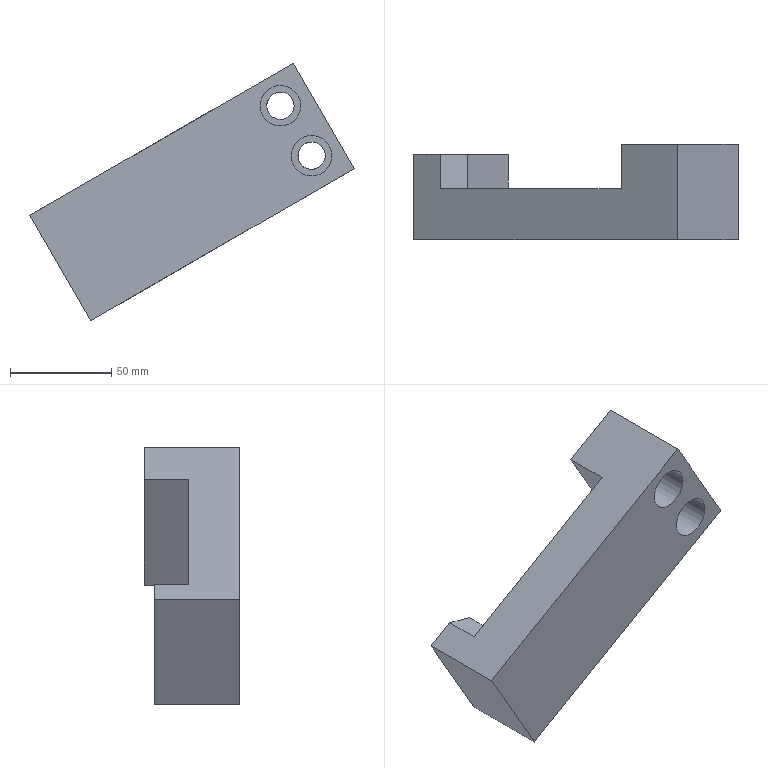Part | NX | features solid 2 | 1 solid | 18 faces | box 159.904 x 47 x 126.962 mm | volume 272454 mm3 | plane 14 | cylinder 4 | commonest cylinder face diameters 13.5 x2 20 x2
STEP:
#1=CARTESIAN_POINT('',(-1100.271,-395.,1.637));
#2=VERTEX_POINT('',#1);
#3=CARTESIAN_POINT('',(-1011.07,-395.,53.137));
#4=VERTEX_POINT('',#3);
#5=CARTESIAN_POINT('',(-1005.874,-395.,56.137));
#6=DIRECTION('',(0.866,0.,0.5));
#7=VECTOR('',#6,1000.);
#8=LINE('',#5,#7);
#9=EDGE_CURVE('',#2,#4,#8,.T.);
#10=ORIENTED_EDGE('',*,*,#9,.T.);
#11=CARTESIAN_POINT('',(-981.07,-395.,1.176));
#12=VERTEX_POINT('',#11);
#13=CARTESIAN_POINT('',(-983.42,-395.,5.246));
#14=DIRECTION('',(-0.5,0.,0.866));
#15=VECTOR('',#14,1000.);
#16=LINE('',#13,#15);
#17=EDGE_CURVE('',#12,#4,#16,.T.);
#18=ORIENTED_EDGE('',*,*,#17,.F.);
#19=CARTESIAN_POINT('',(-1070.271,-395.,-50.324));
#20=VERTEX_POINT('',#19);
#21=CARTESIAN_POINT('',(-975.874,-395.,4.176));
#22=DIRECTION('',(0.866,0.,0.5));
#23=VECTOR('',#22,1000.);
#24=LINE('',#21,#23);
#25=EDGE_CURVE('',#20,#12,#24,.T.);
#26=ORIENTED_EDGE('',*,*,#25,.F.);
#27=CARTESIAN_POINT('',(-1066.61,-395.,-36.664));
#28=VERTEX_POINT('',#27);
#29=CARTESIAN_POINT('',(-1049.462,-395.,27.334));
#30=DIRECTION('',(0.2588,0.,0.9659));
#31=VECTOR('',#30,1000.);
#32=LINE('',#29,#31);
#33=EDGE_CURVE('',#20,#28,#32,.T.);
#34=ORIENTED_EDGE('',*,*,#33,.T.);
#35=CARTESIAN_POINT('',(-1086.61,-395.,-2.023));
#36=VERTEX_POINT('',#35);
#37=CARTESIAN_POINT('',(-1063.96,-395.,-41.254));
#38=DIRECTION('',(-0.5,0.,0.866));
#39=VECTOR('',#38,1000.);
#40=LINE('',#37,#39);
#41=EDGE_CURVE('',#28,#36,#40,.T.);
#42=ORIENTED_EDGE('',*,*,#41,.T.);
#43=CARTESIAN_POINT('',(-988.052,-395.,-28.432));
#44=DIRECTION('',(0.9659,0.,-0.2588));
#45=VECTOR('',#44,1000.);
#46=LINE('',#43,#45);
#47=EDGE_CURVE('',#36,#2,#46,.F.);
#48=ORIENTED_EDGE('',*,*,#47,.T.);
#49=EDGE_LOOP('',(#10,#18,#26,#34,#42,#48));
#50=FACE_BOUND('',#49,.T.);
#51=CARTESIAN_POINT('',(-978.224,-395.,8.246));
#52=DIRECTION('',(0.,1.,0.));
#53=DIRECTION('',(-0.5,0.,0.866));
#54=AXIS2_PLACEMENT_3D('',#51,#52,#53);
#55=PLANE('',#54);
#56=ADVANCED_FACE('',(#50),#55,.T.);
#57=ORIENTED_EDGE('',*,*,#9,.F.);
#58=CARTESIAN_POINT('',(-1100.271,-378.,1.637));
#59=VERTEX_POINT('',#58);
#60=CARTESIAN_POINT('',(-1100.271,-335.,1.637));
#61=DIRECTION('',(0.,-1.,0.));
#62=VECTOR('',#61,1000.);
#63=LINE('',#60,#62);
#64=EDGE_CURVE('',#2,#59,#63,.F.);
#65=ORIENTED_EDGE('',*,*,#64,.T.);
#66=CARTESIAN_POINT('',(-1113.261,-378.,-5.863));
#67=VERTEX_POINT('',#66);
#68=CARTESIAN_POINT('',(-1100.271,-378.,1.637));
#69=DIRECTION('',(0.866,0.,0.5));
#70=VECTOR('',#69,1000.);
#71=LINE('',#68,#70);
#72=EDGE_CURVE('',#67,#59,#71,.T.);
#73=ORIENTED_EDGE('',*,*,#72,.F.);
#74=CARTESIAN_POINT('',(-1113.261,-420.,-5.863));
#75=VERTEX_POINT('',#74);
#76=CARTESIAN_POINT('',(-1113.261,-335.,-5.863));
#77=DIRECTION('',(0.,-1.,0.));
#78=VECTOR('',#77,1000.);
#79=LINE('',#76,#78);
#80=EDGE_CURVE('',#67,#75,#79,.T.);
#81=ORIENTED_EDGE('',*,*,#80,.T.);
#82=CARTESIAN_POINT('',(-983.357,-420.,69.137));
#83=VERTEX_POINT('',#82);
#84=CARTESIAN_POINT('',(-1096.807,-420.,3.637));
#85=DIRECTION('',(0.866,0.,0.5));
#86=VECTOR('',#85,1000.);
#87=LINE('',#84,#86);
#88=EDGE_CURVE('',#75,#83,#87,.T.);
#89=ORIENTED_EDGE('',*,*,#88,.T.);
#90=CARTESIAN_POINT('',(-983.357,-373.,69.137));
#91=VERTEX_POINT('',#90);
#92=CARTESIAN_POINT('',(-983.357,-370.,69.137));
#93=DIRECTION('',(0.,1.,0.));
#94=VECTOR('',#93,1000.);
#95=LINE('',#92,#94);
#96=EDGE_CURVE('',#83,#91,#95,.T.);
#97=ORIENTED_EDGE('',*,*,#96,.T.);
#98=CARTESIAN_POINT('',(-1011.07,-373.,53.137));
#99=VERTEX_POINT('',#98);
#100=CARTESIAN_POINT('',(-1096.807,-373.,3.637));
#101=DIRECTION('',(-0.866,0.,-0.5));
#102=VECTOR('',#101,1000.);
#103=LINE('',#100,#102);
#104=EDGE_CURVE('',#91,#99,#103,.T.);
#105=ORIENTED_EDGE('',*,*,#104,.T.);
#106=CARTESIAN_POINT('',(-1011.07,-335.,53.137));
#107=DIRECTION('',(0.,-1.,0.));
#108=VECTOR('',#107,1000.);
#109=LINE('',#106,#108);
#110=EDGE_CURVE('',#99,#4,#109,.T.);
#111=ORIENTED_EDGE('',*,*,#110,.T.);
#112=EDGE_LOOP('',(#57,#65,#73,#81,#89,#97,#105,#111));
#113=FACE_BOUND('',#112,.T.);
#114=CARTESIAN_POINT('',(-1096.807,-335.,3.637));
#115=DIRECTION('',(-0.5,0.,0.866));
#116=DIRECTION('',(0.866,0.,0.5));
#117=AXIS2_PLACEMENT_3D('',#114,#115,#116);
#118=PLANE('',#117);
#119=ADVANCED_FACE('',(#113),#118,.T.);
#120=ORIENTED_EDGE('',*,*,#72,.T.);
#121=CARTESIAN_POINT('',(-1086.61,-378.,-2.023));
#122=VERTEX_POINT('',#121);
#123=CARTESIAN_POINT('',(-1062.5,-378.,-8.484));
#124=DIRECTION('',(-0.9659,0.,0.2588));
#125=VECTOR('',#124,1000.);
#126=LINE('',#123,#125);
#127=EDGE_CURVE('',#59,#122,#126,.F.);
#128=ORIENTED_EDGE('',*,*,#127,.T.);
#129=CARTESIAN_POINT('',(-1066.61,-378.,-36.664));
#130=VERTEX_POINT('',#129);
#131=CARTESIAN_POINT('',(-1063.96,-378.,-41.254));
#132=DIRECTION('',(-0.5,0.,0.866));
#133=VECTOR('',#132,1000.);
#134=LINE('',#131,#133);
#135=EDGE_CURVE('',#130,#122,#134,.T.);
#136=ORIENTED_EDGE('',*,*,#135,.F.);
#137=CARTESIAN_POINT('',(-1070.271,-378.,-50.324));
#138=VERTEX_POINT('',#137);
#139=CARTESIAN_POINT('',(-1069.411,-378.,-47.114));
#140=DIRECTION('',(-0.2588,0.,-0.9659));
#141=VECTOR('',#140,1000.);
#142=LINE('',#139,#141);
#143=EDGE_CURVE('',#130,#138,#142,.T.);
#144=ORIENTED_EDGE('',*,*,#143,.T.);
#145=CARTESIAN_POINT('',(-1083.261,-378.,-57.824));
#146=VERTEX_POINT('',#145);
#147=CARTESIAN_POINT('',(-1070.271,-378.,-50.324));
#148=DIRECTION('',(0.866,0.,0.5));
#149=VECTOR('',#148,1000.);
#150=LINE('',#147,#149);
#151=EDGE_CURVE('',#146,#138,#150,.T.);
#152=ORIENTED_EDGE('',*,*,#151,.F.);
#153=CARTESIAN_POINT('',(-1085.611,-378.,-53.754));
#154=DIRECTION('',(-0.5,0.,0.866));
#155=VECTOR('',#154,1000.);
#156=LINE('',#153,#155);
#157=EDGE_CURVE('',#146,#67,#156,.T.);
#158=ORIENTED_EDGE('',*,*,#157,.T.);
#159=EDGE_LOOP('',(#120,#128,#136,#144,#152,#158));
#160=FACE_BOUND('',#159,.T.);
#161=CARTESIAN_POINT('',(-1072.621,-378.,-46.254));
#162=DIRECTION('',(0.,1.,0.));
#163=DIRECTION('',(0.342,0.,0.9397));
#164=AXIS2_PLACEMENT_3D('',#161,#162,#163);
#165=PLANE('',#164);
#166=ADVANCED_FACE('',(#160),#165,.T.);
#167=ORIENTED_EDGE('',*,*,#151,.T.);
#168=CARTESIAN_POINT('',(-1070.271,-335.,-50.324));
#169=DIRECTION('',(0.,-1.,0.));
#170=VECTOR('',#169,1000.);
#171=LINE('',#168,#170);
#172=EDGE_CURVE('',#138,#20,#171,.T.);
#173=ORIENTED_EDGE('',*,*,#172,.T.);
#174=ORIENTED_EDGE('',*,*,#25,.T.);
#175=CARTESIAN_POINT('',(-981.07,-373.,1.176));
#176=VERTEX_POINT('',#175);
#177=CARTESIAN_POINT('',(-981.07,-335.,1.176));
#178=DIRECTION('',(0.,-1.,0.));
#179=VECTOR('',#178,1000.);
#180=LINE('',#177,#179);
#181=EDGE_CURVE('',#176,#12,#180,.T.);
#182=ORIENTED_EDGE('',*,*,#181,.F.);
#183=CARTESIAN_POINT('',(-953.357,-373.,17.176));
#184=VERTEX_POINT('',#183);
#185=CARTESIAN_POINT('',(-1066.807,-373.,-48.324));
#186=DIRECTION('',(-0.866,0.,-0.5));
#187=VECTOR('',#186,1000.);
#188=LINE('',#185,#187);
#189=EDGE_CURVE('',#184,#176,#188,.T.);
#190=ORIENTED_EDGE('',*,*,#189,.F.);
#191=CARTESIAN_POINT('',(-953.357,-420.,17.176));
#192=VERTEX_POINT('',#191);
#193=CARTESIAN_POINT('',(-953.357,-370.,17.176));
#194=DIRECTION('',(0.,1.,0.));
#195=VECTOR('',#194,1000.);
#196=LINE('',#193,#195);
#197=EDGE_CURVE('',#192,#184,#196,.T.);
#198=ORIENTED_EDGE('',*,*,#197,.F.);
#199=CARTESIAN_POINT('',(-1083.261,-420.,-57.824));
#200=VERTEX_POINT('',#199);
#201=CARTESIAN_POINT('',(-1066.807,-420.,-48.324));
#202=DIRECTION('',(0.866,0.,0.5));
#203=VECTOR('',#202,1000.);
#204=LINE('',#201,#203);
#205=EDGE_CURVE('',#200,#192,#204,.T.);
#206=ORIENTED_EDGE('',*,*,#205,.F.);
#207=CARTESIAN_POINT('',(-1083.261,-335.,-57.824));
#208=DIRECTION('',(0.,-1.,0.));
#209=VECTOR('',#208,1000.);
#210=LINE('',#207,#209);
#211=EDGE_CURVE('',#146,#200,#210,.T.);
#212=ORIENTED_EDGE('',*,*,#211,.F.);
#213=EDGE_LOOP('',(#167,#173,#174,#182,#190,#198,#206,#212));
#214=FACE_BOUND('',#213,.T.);
#215=CARTESIAN_POINT('',(-1066.807,-335.,-48.324));
#216=DIRECTION('',(-0.5,0.,0.866));
#217=DIRECTION('',(0.866,0.,0.5));
#218=AXIS2_PLACEMENT_3D('',#215,#216,#217);
#219=PLANE('',#218);
#220=ADVANCED_FACE('',(#214),#219,.F.);
#221=CARTESIAN_POINT('',(-970.927,-420.,32.929));
#222=VERTEX_POINT('',#221);
#223=CARTESIAN_POINT('',(-974.348,-420.,23.532));
#224=DIRECTION('',(0.,1.,0.));
#225=DIRECTION('',(0.342,0.,0.9397));
#226=AXIS2_PLACEMENT_3D('',#223,#224,#225);
#227=CIRCLE('',#226,10.);
#228=EDGE_CURVE('',#222,#222,#227,.T.);
#229=ORIENTED_EDGE('',*,*,#228,.T.);
#230=EDGE_LOOP('',(#229));
#231=FACE_BOUND('',#230,.T.);
#232=CARTESIAN_POINT('',(-986.293,-420.,57.544));
#233=VERTEX_POINT('',#232);
#234=CARTESIAN_POINT('',(-989.714,-420.,48.147));
#235=DIRECTION('',(0.,1.,0.));
#236=DIRECTION('',(0.342,0.,0.9397));
#237=AXIS2_PLACEMENT_3D('',#234,#235,#236);
#238=CIRCLE('',#237,10.);
#239=EDGE_CURVE('',#233,#233,#238,.T.);
#240=ORIENTED_EDGE('',*,*,#239,.T.);
#241=EDGE_LOOP('',(#240));
#242=FACE_BOUND('',#241,.T.);
#243=ORIENTED_EDGE('',*,*,#205,.T.);
#244=CARTESIAN_POINT('',(-955.707,-420.,21.246));
#245=DIRECTION('',(-0.5,0.,0.866));
#246=VECTOR('',#245,1000.);
#247=LINE('',#244,#246);
#248=EDGE_CURVE('',#192,#83,#247,.T.);
#249=ORIENTED_EDGE('',*,*,#248,.T.);
#250=ORIENTED_EDGE('',*,*,#88,.F.);
#251=CARTESIAN_POINT('',(-1085.611,-420.,-53.754));
#252=DIRECTION('',(-0.5,0.,0.866));
#253=VECTOR('',#252,1000.);
#254=LINE('',#251,#253);
#255=EDGE_CURVE('',#200,#75,#254,.T.);
#256=ORIENTED_EDGE('',*,*,#255,.F.);
#257=EDGE_LOOP('',(#243,#249,#250,#256));
#258=FACE_BOUND('',#257,.T.);
#259=CARTESIAN_POINT('',(-1069.157,-420.,-44.254));
#260=DIRECTION('',(0.,1.,0.));
#261=DIRECTION('',(0.342,0.,0.9397));
#262=AXIS2_PLACEMENT_3D('',#259,#260,#261);
#263=PLANE('',#262);
#264=ADVANCED_FACE('',(#231,#242,#258),#263,.F.);
#265=ORIENTED_EDGE('',*,*,#211,.T.);
#266=ORIENTED_EDGE('',*,*,#255,.T.);
#267=ORIENTED_EDGE('',*,*,#80,.F.);
#268=ORIENTED_EDGE('',*,*,#157,.F.);
#269=EDGE_LOOP('',(#265,#266,#267,#268));
#270=FACE_BOUND('',#269,.T.);
#271=CARTESIAN_POINT('',(-1085.611,-335.,-53.754));
#272=DIRECTION('',(0.866,0.,0.5));
#273=DIRECTION('',(0.5,0.,-0.866));
#274=AXIS2_PLACEMENT_3D('',#271,#272,#273);
#275=PLANE('',#274);
#276=ADVANCED_FACE('',(#270),#275,.F.);
#277=ORIENTED_EDGE('',*,*,#135,.T.);
#278=CARTESIAN_POINT('',(-1086.61,-335.,-2.023));
#279=DIRECTION('',(0.,-1.,0.));
#280=VECTOR('',#279,1000.);
#281=LINE('',#278,#280);
#282=EDGE_CURVE('',#122,#36,#281,.T.);
#283=ORIENTED_EDGE('',*,*,#282,.T.);
#284=ORIENTED_EDGE('',*,*,#41,.F.);
#285=CARTESIAN_POINT('',(-1066.61,-380.,-36.664));
#286=DIRECTION('',(0.,1.,0.));
#287=VECTOR('',#286,1000.);
#288=LINE('',#285,#287);
#289=EDGE_CURVE('',#28,#130,#288,.T.);
#290=ORIENTED_EDGE('',*,*,#289,.T.);
#291=EDGE_LOOP('',(#277,#283,#284,#290));
#292=FACE_BOUND('',#291,.T.);
#293=CARTESIAN_POINT('',(-1063.96,-335.,-41.254));
#294=DIRECTION('',(0.866,0.,0.5));
#295=DIRECTION('',(0.5,0.,-0.866));
#296=AXIS2_PLACEMENT_3D('',#293,#294,#295);
#297=PLANE('',#296);
#298=ADVANCED_FACE('',(#292),#297,.T.);
#299=ORIENTED_EDGE('',*,*,#197,.T.);
#300=CARTESIAN_POINT('',(-955.707,-373.,21.246));
#301=DIRECTION('',(-0.5,0.,0.866));
#302=VECTOR('',#301,1000.);
#303=LINE('',#300,#302);
#304=EDGE_CURVE('',#184,#91,#303,.T.);
#305=ORIENTED_EDGE('',*,*,#304,.T.);
#306=ORIENTED_EDGE('',*,*,#96,.F.);
#307=ORIENTED_EDGE('',*,*,#248,.F.);
#308=EDGE_LOOP('',(#299,#305,#306,#307));
#309=FACE_BOUND('',#308,.T.);
#310=CARTESIAN_POINT('',(-955.707,-370.,21.246));
#311=DIRECTION('',(-0.866,0.,-0.5));
#312=DIRECTION('',(-0.5,0.,0.866));
#313=AXIS2_PLACEMENT_3D('',#310,#311,#312);
#314=PLANE('',#313);
#315=ADVANCED_FACE('',(#309),#314,.F.);
#316=CARTESIAN_POINT('',(-974.348,-373.,30.282));
#317=VERTEX_POINT('',#316);
#318=CARTESIAN_POINT('',(-974.348,-373.,23.532));
#319=DIRECTION('',(0.,1.,0.));
#320=DIRECTION('',(0.,0.,1.));
#321=AXIS2_PLACEMENT_3D('',#318,#319,#320);
#322=CIRCLE('',#321,6.75);
#323=EDGE_CURVE('',#317,#317,#322,.T.);
#324=ORIENTED_EDGE('',*,*,#323,.F.);
#325=EDGE_LOOP('',(#324));
#326=FACE_BOUND('',#325,.T.);
#327=CARTESIAN_POINT('',(-989.714,-373.,54.897));
#328=VERTEX_POINT('',#327);
#329=CARTESIAN_POINT('',(-989.714,-373.,48.147));
#330=DIRECTION('',(0.,1.,0.));
#331=DIRECTION('',(0.,0.,1.));
#332=AXIS2_PLACEMENT_3D('',#329,#330,#331);
#333=CIRCLE('',#332,6.75);
#334=EDGE_CURVE('',#328,#328,#333,.T.);
#335=ORIENTED_EDGE('',*,*,#334,.F.);
#336=EDGE_LOOP('',(#335));
#337=FACE_BOUND('',#336,.T.);
#338=ORIENTED_EDGE('',*,*,#104,.F.);
#339=ORIENTED_EDGE('',*,*,#304,.F.);
#340=ORIENTED_EDGE('',*,*,#189,.T.);
#341=CARTESIAN_POINT('',(-982.32,-373.,3.341));
#342=DIRECTION('',(-0.5,0.,0.866));
#343=VECTOR('',#342,1000.);
#344=LINE('',#341,#343);
#345=EDGE_CURVE('',#176,#99,#344,.T.);
#346=ORIENTED_EDGE('',*,*,#345,.T.);
#347=EDGE_LOOP('',(#338,#339,#340,#346));
#348=FACE_BOUND('',#347,.T.);
#349=CARTESIAN_POINT('',(-1082.147,-373.,-51.754));
#350=DIRECTION('',(0.,1.,0.));
#351=DIRECTION('',(0.342,0.,0.9397));
#352=AXIS2_PLACEMENT_3D('',#349,#350,#351);
#353=PLANE('',#352);
#354=ADVANCED_FACE('',(#326,#337,#348),#353,.T.);
#355=ORIENTED_EDGE('',*,*,#17,.T.);
#356=ORIENTED_EDGE('',*,*,#110,.F.);
#357=ORIENTED_EDGE('',*,*,#345,.F.);
#358=ORIENTED_EDGE('',*,*,#181,.T.);
#359=EDGE_LOOP('',(#355,#356,#357,#358));
#360=FACE_BOUND('',#359,.T.);
#361=CARTESIAN_POINT('',(-982.32,-380.,3.341));
#362=DIRECTION('',(0.866,0.,0.5));
#363=DIRECTION('',(0.5,0.,-0.866));
#364=AXIS2_PLACEMENT_3D('',#361,#362,#363);
#365=PLANE('',#364);
#366=ADVANCED_FACE('',(#360),#365,.F.);
#367=ORIENTED_EDGE('',*,*,#334,.T.);
#368=EDGE_LOOP('',(#367));
#369=FACE_BOUND('',#368,.T.);
#370=CARTESIAN_POINT('',(-987.405,-405.,54.49));
#371=VERTEX_POINT('',#370);
#372=CARTESIAN_POINT('',(-989.714,-405.,48.147));
#373=DIRECTION('',(0.,1.,0.));
#374=DIRECTION('',(0.342,0.,0.9397));
#375=AXIS2_PLACEMENT_3D('',#372,#373,#374);
#376=CIRCLE('',#375,6.75);
#377=EDGE_CURVE('',#371,#371,#376,.T.);
#378=ORIENTED_EDGE('',*,*,#377,.F.);
#379=EDGE_LOOP('',(#378));
#380=FACE_BOUND('',#379,.T.);
#381=CARTESIAN_POINT('',(-989.714,-370.,48.147));
#382=DIRECTION('',(0.,1.,0.));
#383=DIRECTION('',(0.342,0.,0.9397));
#384=AXIS2_PLACEMENT_3D('',#381,#382,#383);
#385=CYLINDRICAL_SURFACE('',#384,6.75);
#386=ADVANCED_FACE('',(#369,#380),#385,.F.);
#387=ORIENTED_EDGE('',*,*,#377,.T.);
#388=EDGE_LOOP('',(#387));
#389=FACE_BOUND('',#388,.T.);
#390=CARTESIAN_POINT('',(-986.293,-405.,57.544));
#391=VERTEX_POINT('',#390);
#392=CARTESIAN_POINT('',(-989.714,-405.,48.147));
#393=DIRECTION('',(0.,1.,0.));
#394=DIRECTION('',(0.342,0.,0.9397));
#395=AXIS2_PLACEMENT_3D('',#392,#393,#394);
#396=CIRCLE('',#395,10.);
#397=EDGE_CURVE('',#391,#391,#396,.T.);
#398=ORIENTED_EDGE('',*,*,#397,.F.);
#399=EDGE_LOOP('',(#398));
#400=FACE_BOUND('',#399,.T.);
#401=CARTESIAN_POINT('',(-989.714,-405.,48.147));
#402=DIRECTION('',(0.,1.,0.));
#403=DIRECTION('',(0.342,0.,0.9397));
#404=AXIS2_PLACEMENT_3D('',#401,#402,#403);
#405=PLANE('',#404);
#406=ADVANCED_FACE('',(#389,#400),#405,.F.);
#407=ORIENTED_EDGE('',*,*,#397,.T.);
#408=EDGE_LOOP('',(#407));
#409=FACE_BOUND('',#408,.T.);
#410=ORIENTED_EDGE('',*,*,#239,.F.);
#411=EDGE_LOOP('',(#410));
#412=FACE_BOUND('',#411,.T.);
#413=CARTESIAN_POINT('',(-989.714,-420.,48.147));
#414=DIRECTION('',(0.,1.,0.));
#415=DIRECTION('',(0.342,0.,0.9397));
#416=AXIS2_PLACEMENT_3D('',#413,#414,#415);
#417=CYLINDRICAL_SURFACE('',#416,10.);
#418=ADVANCED_FACE('',(#409,#412),#417,.F.);
#419=ORIENTED_EDGE('',*,*,#323,.T.);
#420=EDGE_LOOP('',(#419));
#421=FACE_BOUND('',#420,.T.);
#422=CARTESIAN_POINT('',(-972.039,-405.,29.875));
#423=VERTEX_POINT('',#422);
#424=CARTESIAN_POINT('',(-974.348,-405.,23.532));
#425=DIRECTION('',(0.,1.,0.));
#426=DIRECTION('',(0.342,0.,0.9397));
#427=AXIS2_PLACEMENT_3D('',#424,#425,#426);
#428=CIRCLE('',#427,6.75);
#429=EDGE_CURVE('',#423,#423,#428,.T.);
#430=ORIENTED_EDGE('',*,*,#429,.F.);
#431=EDGE_LOOP('',(#430));
#432=FACE_BOUND('',#431,.T.);
#433=CARTESIAN_POINT('',(-974.348,-370.,23.532));
#434=DIRECTION('',(0.,1.,0.));
#435=DIRECTION('',(0.342,0.,0.9397));
#436=AXIS2_PLACEMENT_3D('',#433,#434,#435);
#437=CYLINDRICAL_SURFACE('',#436,6.75);
#438=ADVANCED_FACE('',(#421,#432),#437,.F.);
#439=ORIENTED_EDGE('',*,*,#429,.T.);
#440=EDGE_LOOP('',(#439));
#441=FACE_BOUND('',#440,.T.);
#442=CARTESIAN_POINT('',(-970.927,-405.,32.929));
#443=VERTEX_POINT('',#442);
#444=CARTESIAN_POINT('',(-974.348,-405.,23.532));
#445=DIRECTION('',(0.,1.,0.));
#446=DIRECTION('',(0.342,0.,0.9397));
#447=AXIS2_PLACEMENT_3D('',#444,#445,#446);
#448=CIRCLE('',#447,10.);
#449=EDGE_CURVE('',#443,#443,#448,.T.);
#450=ORIENTED_EDGE('',*,*,#449,.F.);
#451=EDGE_LOOP('',(#450));
#452=FACE_BOUND('',#451,.T.);
#453=CARTESIAN_POINT('',(-974.348,-405.,23.532));
#454=DIRECTION('',(0.,1.,0.));
#455=DIRECTION('',(0.342,0.,0.9397));
#456=AXIS2_PLACEMENT_3D('',#453,#454,#455);
#457=PLANE('',#456);
#458=ADVANCED_FACE('',(#441,#452),#457,.F.);
#459=ORIENTED_EDGE('',*,*,#449,.T.);
#460=EDGE_LOOP('',(#459));
#461=FACE_BOUND('',#460,.T.);
#462=ORIENTED_EDGE('',*,*,#228,.F.);
#463=EDGE_LOOP('',(#462));
#464=FACE_BOUND('',#463,.T.);
#465=CARTESIAN_POINT('',(-974.348,-420.,23.532));
#466=DIRECTION('',(0.,1.,0.));
#467=DIRECTION('',(0.342,0.,0.9397));
#468=AXIS2_PLACEMENT_3D('',#465,#466,#467);
#469=CYLINDRICAL_SURFACE('',#468,10.);
#470=ADVANCED_FACE('',(#461,#464),#469,.F.);
#471=ORIENTED_EDGE('',*,*,#127,.F.);
#472=ORIENTED_EDGE('',*,*,#64,.F.);
#473=ORIENTED_EDGE('',*,*,#47,.F.);
#474=ORIENTED_EDGE('',*,*,#282,.F.);
#475=EDGE_LOOP('',(#471,#472,#473,#474));
#476=FACE_BOUND('',#475,.T.);
#477=CARTESIAN_POINT('',(-1086.61,-335.,-2.023));
#478=DIRECTION('',(-0.2588,0.,-0.9659));
#479=DIRECTION('',(-0.9659,0.,0.2588));
#480=AXIS2_PLACEMENT_3D('',#477,#478,#479);
#481=PLANE('',#480);
#482=ADVANCED_FACE('',(#476),#481,.F.);
#483=ORIENTED_EDGE('',*,*,#143,.F.);
#484=ORIENTED_EDGE('',*,*,#289,.F.);
#485=ORIENTED_EDGE('',*,*,#33,.F.);
#486=ORIENTED_EDGE('',*,*,#172,.F.);
#487=EDGE_LOOP('',(#483,#484,#485,#486));
#488=FACE_BOUND('',#487,.T.);
#489=CARTESIAN_POINT('',(-1070.271,-335.,-50.324));
#490=DIRECTION('',(0.9659,0.,-0.2588));
#491=DIRECTION('',(-0.2588,0.,-0.9659));
#492=AXIS2_PLACEMENT_3D('',#489,#490,#491);
#493=PLANE('',#492);
#494=ADVANCED_FACE('',(#488),#493,.T.);
#495=CLOSED_SHELL('',(#56,#119,#166,#220,#264,#276,#298,#315,#354,#366,#386,#406,#418,#438,#458,#470,#482,#494));
#496=MANIFOLD_SOLID_BREP('',#495);
#497=(LENGTH_UNIT()NAMED_UNIT(*)SI_UNIT(.MILLI.,.METRE.));
#498=UNCERTAINTY_MEASURE_WITH_UNIT(LENGTH_MEASURE(0.00001),#497,'','');
#499=(NAMED_UNIT(*)PLANE_ANGLE_UNIT()SI_UNIT($,.RADIAN.));
#500=(NAMED_UNIT(*)SI_UNIT($,.STERADIAN.)SOLID_ANGLE_UNIT());
#501=(GEOMETRIC_REPRESENTATION_CONTEXT(3)GLOBAL_UNCERTAINTY_ASSIGNED_CONTEXT((#498))GLOBAL_UNIT_ASSIGNED_CONTEXT((#497,#499,#500))REPRESENTATION_CONTEXT('',''));
#502=ADVANCED_BREP_SHAPE_REPRESENTATION('',(#496),#501);